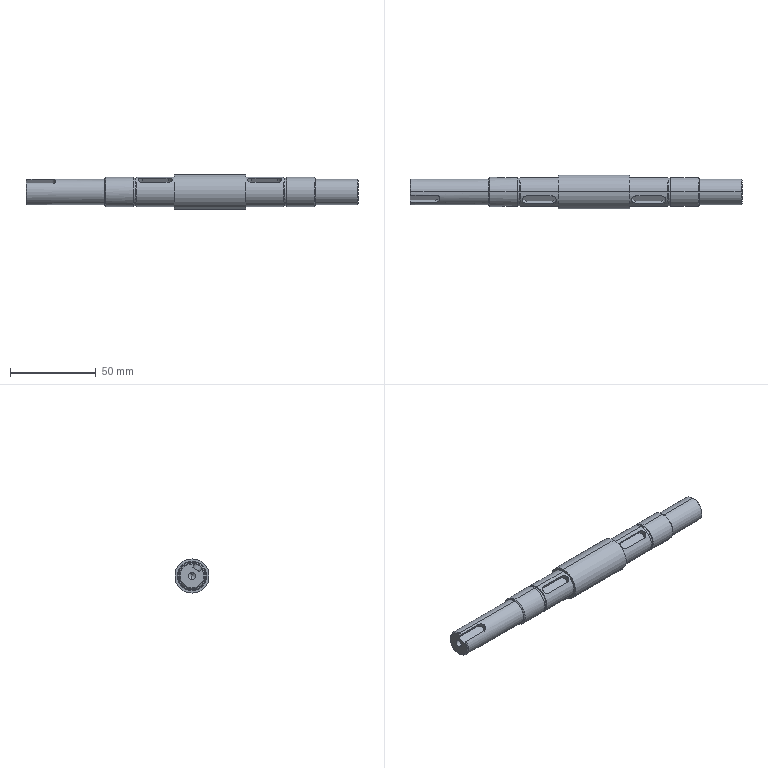Part | SolidWorks | features BaseBody 1 | 1 solid | 63 faces | box 194 x 20 x 20 mm | volume 43037 mm3 | cylinder 25 | plane 19 | cone 11 | spline 8 | commonest cylinder face diameters 17 x8 5 x5 15 x4 16 x4 4.2 x2 20 x2